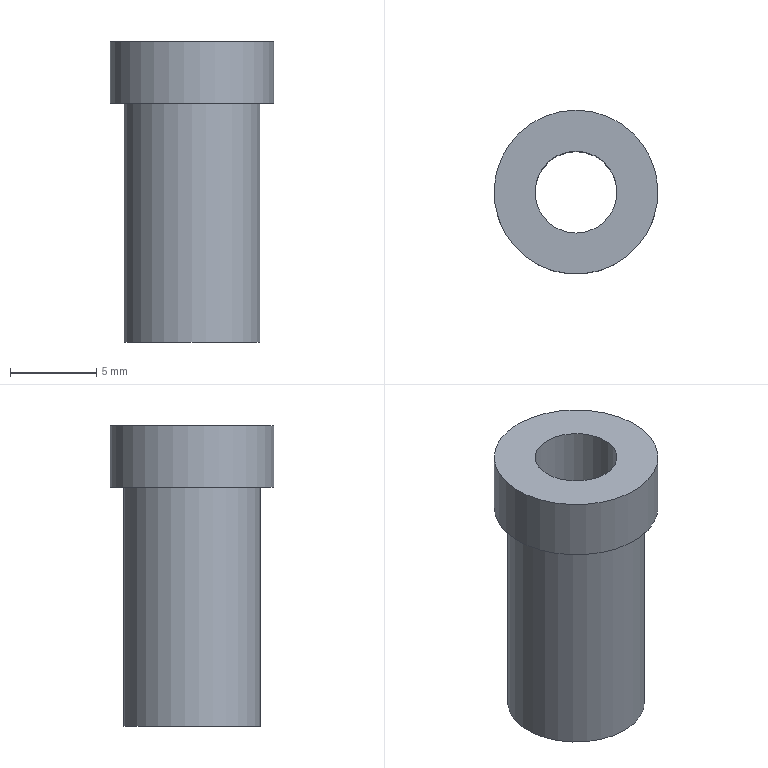Part | NX | features DATUM_CSYS 2, SKETCH 1, SWP104 1 | 1 solid | 6 faces | box 9.525 x 9.525 x 17.463 mm | volume 630.793 mm3 | plane 3 | cylinder 3 | commonest cylinder face diameters 4.762 x1 7.937 x1 9.525 x1
STEP:
#1=CARTESIAN_POINT('',(0.,3.969,0.));
#2=VERTEX_POINT('',#1);
#3=CARTESIAN_POINT('',(0.,0.,0.));
#4=DIRECTION('',(0.,0.,-1.));
#5=DIRECTION('',(0.,1.,0.));
#6=AXIS2_PLACEMENT_3D('',#3,#4,#5);
#7=CIRCLE('',#6,3.969);
#8=EDGE_CURVE('',#2,#2,#7,.T.);
#9=ORIENTED_EDGE('',*,*,#8,.T.);
#10=EDGE_LOOP('',(#9));
#11=FACE_BOUND('',#10,.T.);
#12=CARTESIAN_POINT('',(0.,2.381,0.));
#13=VERTEX_POINT('',#12);
#14=CARTESIAN_POINT('',(0.,0.,0.));
#15=DIRECTION('',(0.,0.,-1.));
#16=DIRECTION('',(0.,1.,0.));
#17=AXIS2_PLACEMENT_3D('',#14,#15,#16);
#18=CIRCLE('',#17,2.381);
#19=EDGE_CURVE('',#13,#13,#18,.T.);
#20=ORIENTED_EDGE('',*,*,#19,.F.);
#21=EDGE_LOOP('',(#20));
#22=FACE_BOUND('',#21,.T.);
#23=CARTESIAN_POINT('',(0.,2.381,0.));
#24=DIRECTION('',(0.,0.,-1.));
#25=DIRECTION('',(0.,1.,0.));
#26=AXIS2_PLACEMENT_3D('',#23,#24,#25);
#27=PLANE('',#26);
#28=ADVANCED_FACE('',(#11,#22),#27,.T.);
#29=CARTESIAN_POINT('',(0.,3.969,13.891));
#30=VERTEX_POINT('',#29);
#31=CARTESIAN_POINT('',(0.,0.,13.891));
#32=DIRECTION('',(0.,0.,-1.));
#33=DIRECTION('',(0.,1.,0.));
#34=AXIS2_PLACEMENT_3D('',#31,#32,#33);
#35=CIRCLE('',#34,3.969);
#36=EDGE_CURVE('',#30,#30,#35,.T.);
#37=ORIENTED_EDGE('',*,*,#36,.T.);
#38=EDGE_LOOP('',(#37));
#39=FACE_BOUND('',#38,.T.);
#40=ORIENTED_EDGE('',*,*,#8,.F.);
#41=EDGE_LOOP('',(#40));
#42=FACE_BOUND('',#41,.T.);
#43=CARTESIAN_POINT('',(0.,0.,0.));
#44=DIRECTION('',(0.,0.,-1.));
#45=DIRECTION('',(0.,1.,0.));
#46=AXIS2_PLACEMENT_3D('',#43,#44,#45);
#47=CYLINDRICAL_SURFACE('',#46,3.969);
#48=ADVANCED_FACE('',(#39,#42),#47,.T.);
#49=CARTESIAN_POINT('',(0.,4.763,13.891));
#50=VERTEX_POINT('',#49);
#51=CARTESIAN_POINT('',(0.,0.,13.891));
#52=DIRECTION('',(0.,0.,-1.));
#53=DIRECTION('',(0.,1.,0.));
#54=AXIS2_PLACEMENT_3D('',#51,#52,#53);
#55=CIRCLE('',#54,4.762);
#56=EDGE_CURVE('',#50,#50,#55,.T.);
#57=ORIENTED_EDGE('',*,*,#56,.T.);
#58=EDGE_LOOP('',(#57));
#59=FACE_BOUND('',#58,.T.);
#60=ORIENTED_EDGE('',*,*,#36,.F.);
#61=EDGE_LOOP('',(#60));
#62=FACE_BOUND('',#61,.T.);
#63=CARTESIAN_POINT('',(0.,3.969,13.891));
#64=DIRECTION('',(0.,0.,-1.));
#65=DIRECTION('',(0.,1.,0.));
#66=AXIS2_PLACEMENT_3D('',#63,#64,#65);
#67=PLANE('',#66);
#68=ADVANCED_FACE('',(#59,#62),#67,.T.);
#69=CARTESIAN_POINT('',(0.,4.763,17.462));
#70=VERTEX_POINT('',#69);
#71=CARTESIAN_POINT('',(0.,0.,17.462));
#72=DIRECTION('',(0.,0.,-1.));
#73=DIRECTION('',(0.,1.,0.));
#74=AXIS2_PLACEMENT_3D('',#71,#72,#73);
#75=CIRCLE('',#74,4.762);
#76=EDGE_CURVE('',#70,#70,#75,.T.);
#77=ORIENTED_EDGE('',*,*,#76,.T.);
#78=EDGE_LOOP('',(#77));
#79=FACE_BOUND('',#78,.T.);
#80=ORIENTED_EDGE('',*,*,#56,.F.);
#81=EDGE_LOOP('',(#80));
#82=FACE_BOUND('',#81,.T.);
#83=CARTESIAN_POINT('',(0.,0.,0.));
#84=DIRECTION('',(0.,0.,-1.));
#85=DIRECTION('',(0.,1.,0.));
#86=AXIS2_PLACEMENT_3D('',#83,#84,#85);
#87=CYLINDRICAL_SURFACE('',#86,4.762);
#88=ADVANCED_FACE('',(#79,#82),#87,.T.);
#89=CARTESIAN_POINT('',(0.,2.381,17.462));
#90=VERTEX_POINT('',#89);
#91=CARTESIAN_POINT('',(0.,0.,17.462));
#92=DIRECTION('',(0.,0.,-1.));
#93=DIRECTION('',(0.,1.,0.));
#94=AXIS2_PLACEMENT_3D('',#91,#92,#93);
#95=CIRCLE('',#94,2.381);
#96=EDGE_CURVE('',#90,#90,#95,.T.);
#97=ORIENTED_EDGE('',*,*,#96,.T.);
#98=EDGE_LOOP('',(#97));
#99=FACE_BOUND('',#98,.T.);
#100=ORIENTED_EDGE('',*,*,#76,.F.);
#101=EDGE_LOOP('',(#100));
#102=FACE_BOUND('',#101,.T.);
#103=CARTESIAN_POINT('',(0.,4.763,17.462));
#104=DIRECTION('',(0.,0.,1.));
#105=DIRECTION('',(0.,-1.,0.));
#106=AXIS2_PLACEMENT_3D('',#103,#104,#105);
#107=PLANE('',#106);
#108=ADVANCED_FACE('',(#99,#102),#107,.T.);
#109=ORIENTED_EDGE('',*,*,#19,.T.);
#110=EDGE_LOOP('',(#109));
#111=FACE_BOUND('',#110,.T.);
#112=ORIENTED_EDGE('',*,*,#96,.F.);
#113=EDGE_LOOP('',(#112));
#114=FACE_BOUND('',#113,.T.);
#115=CARTESIAN_POINT('',(0.,0.,0.));
#116=DIRECTION('',(0.,0.,-1.));
#117=DIRECTION('',(0.,1.,0.));
#118=AXIS2_PLACEMENT_3D('',#115,#116,#117);
#119=CYLINDRICAL_SURFACE('',#118,2.381);
#120=ADVANCED_FACE('',(#111,#114),#119,.F.);
#121=CLOSED_SHELL('',(#28,#48,#68,#88,#108,#120));
#122=MANIFOLD_SOLID_BREP('',#121);
#123=(LENGTH_UNIT()NAMED_UNIT(*)SI_UNIT(.MILLI.,.METRE.));
#124=UNCERTAINTY_MEASURE_WITH_UNIT(LENGTH_MEASURE(0.00001),#123,'','');
#125=(NAMED_UNIT(*)PLANE_ANGLE_UNIT()SI_UNIT($,.RADIAN.));
#126=(NAMED_UNIT(*)SI_UNIT($,.STERADIAN.)SOLID_ANGLE_UNIT());
#127=(GEOMETRIC_REPRESENTATION_CONTEXT(3)GLOBAL_UNCERTAINTY_ASSIGNED_CONTEXT((#124))GLOBAL_UNIT_ASSIGNED_CONTEXT((#123,#125,#126))REPRESENTATION_CONTEXT('',''));
#128=ADVANCED_BREP_SHAPE_REPRESENTATION('',(#122),#127);